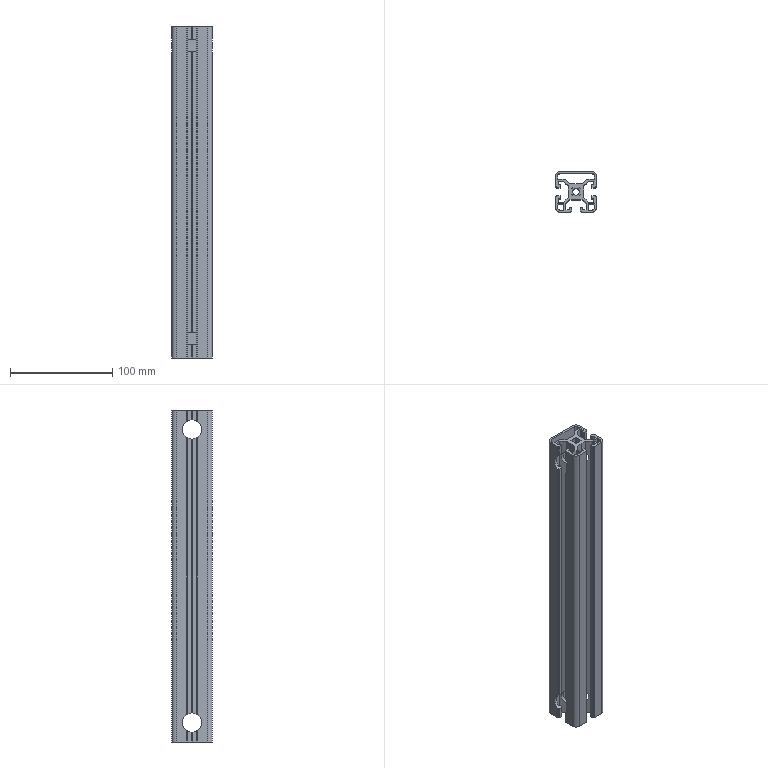Part | SolidWorks | features BaseBody 1, HoleWzd 1, MoveFace 1 | 1 solid | 242 faces | box 40 x 40 x 325 mm | volume 184039 mm3 | plane 187 | cylinder 55 | commonest cylinder face diameters 6.8 x15 2 x14 19 x12 1 x6 5 x4 9 x4